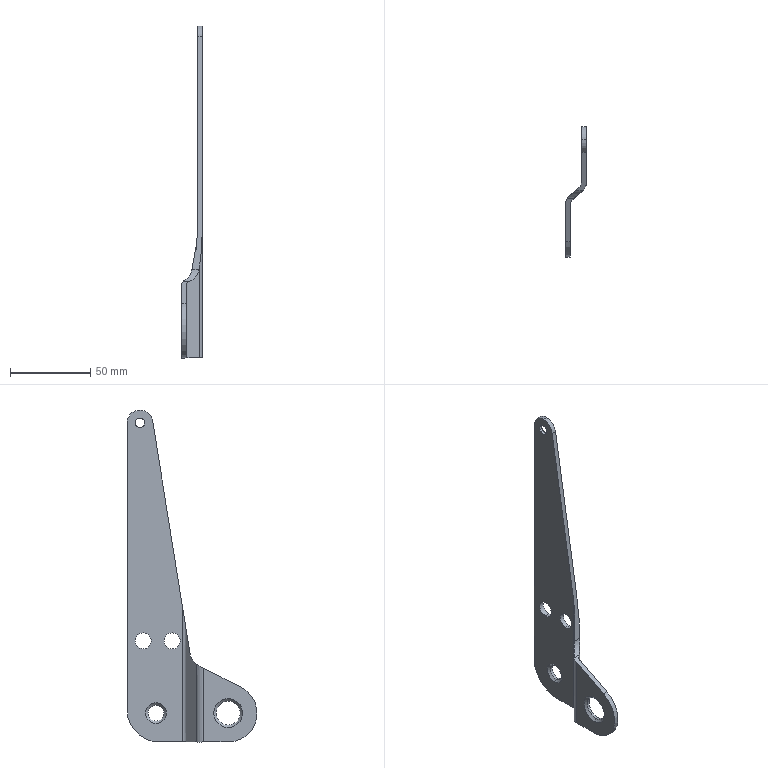Part | STEP file | 8XS174010 | 1 solid | 35 faces | box 13 x 81 x 207 mm | volume 22375 mm3 | cylinder 19 | plane 10 | cone 6 | commonest cylinder face diameters 10 x6 6 x4 12 x2 15 x2 16 x2 20 x1